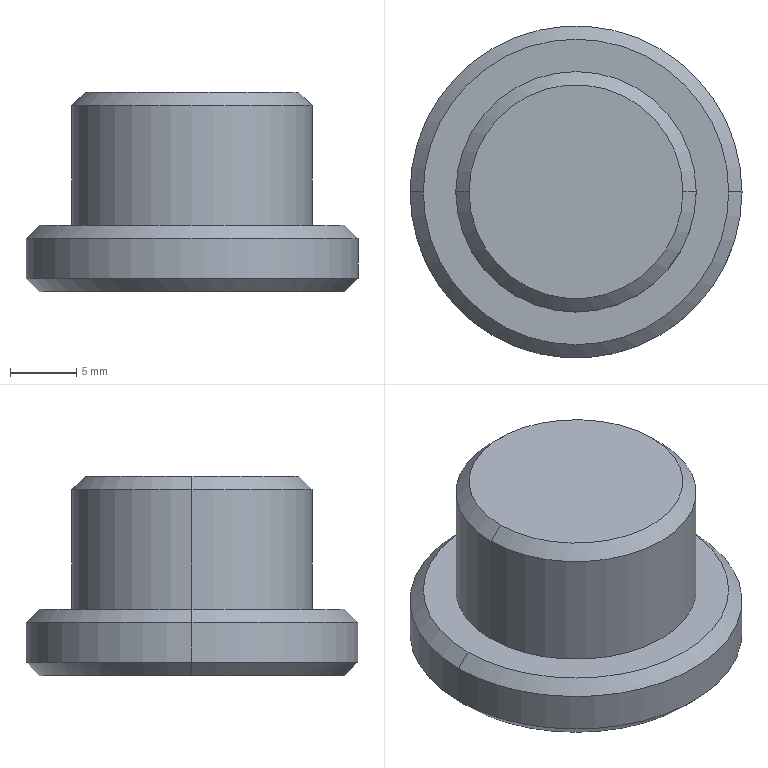Part | SolidWorks | features Chamfer 1, Revolution 1 | 1 solid | 13 faces | box 25 x 25 x 15 mm | volume 4924 mm3 | cone 6 | cylinder 4 | plane 3 | commonest cylinder face diameters 18.1 x2 25 x2
STEP:
#1=CARTESIAN_POINT('',(8.05,0.,0.));
#2=VERTEX_POINT('',#1);
#3=CARTESIAN_POINT('',(-8.05,0.,0.));
#4=VERTEX_POINT('',#3);
#5=CARTESIAN_POINT('',(0.,0.,0.));
#6=DIRECTION('',(0.,0.,1.));
#7=DIRECTION('',(-1.,0.,0.));
#8=AXIS2_PLACEMENT_3D('',#5,#6,#7);
#9=CIRCLE('',#8,8.05);
#10=EDGE_CURVE('',#2,#4,#9,.T.);
#11=ORIENTED_EDGE('',*,*,#10,.F.);
#12=CARTESIAN_POINT('',(9.05,0.,-1.));
#13=VERTEX_POINT('',#12);
#14=CARTESIAN_POINT('',(8.05,0.,0.));
#15=DIRECTION('',(0.7071,0.,-0.7071));
#16=VECTOR('',#15,1000.);
#17=LINE('',#14,#16);
#18=EDGE_CURVE('',#2,#13,#17,.T.);
#19=ORIENTED_EDGE('',*,*,#18,.T.);
#20=CARTESIAN_POINT('',(-9.05,0.,-1.));
#21=VERTEX_POINT('',#20);
#22=CARTESIAN_POINT('',(0.,0.,-1.));
#23=DIRECTION('',(0.,0.,-1.));
#24=DIRECTION('',(-1.,0.,0.));
#25=AXIS2_PLACEMENT_3D('',#22,#23,#24);
#26=CIRCLE('',#25,9.05);
#27=EDGE_CURVE('',#21,#13,#26,.T.);
#28=ORIENTED_EDGE('',*,*,#27,.F.);
#29=CARTESIAN_POINT('',(-8.05,0.,0.));
#30=DIRECTION('',(-0.7071,0.,-0.7071));
#31=VECTOR('',#30,1000.);
#32=LINE('',#29,#31);
#33=EDGE_CURVE('',#4,#21,#32,.T.);
#34=ORIENTED_EDGE('',*,*,#33,.F.);
#35=EDGE_LOOP('',(#11,#19,#28,#34));
#36=FACE_OUTER_BOUND('',#35,.T.);
#37=CARTESIAN_POINT('',(0.,0.,0.));
#38=DIRECTION('',(0.,0.,-1.));
#39=DIRECTION('',(-1.,0.,0.));
#40=AXIS2_PLACEMENT_3D('',#37,#38,#39);
#41=CONICAL_SURFACE('',#40,8.05,0.7854);
#42=ADVANCED_FACE('',(#36),#41,.T.);
#43=CARTESIAN_POINT('',(11.5,0.,-10.));
#44=VERTEX_POINT('',#43);
#45=CARTESIAN_POINT('',(-11.5,0.,-10.));
#46=VERTEX_POINT('',#45);
#47=CARTESIAN_POINT('',(0.,0.,-10.));
#48=DIRECTION('',(0.,0.,1.));
#49=DIRECTION('',(-1.,0.,0.));
#50=AXIS2_PLACEMENT_3D('',#47,#48,#49);
#51=CIRCLE('',#50,11.5);
#52=EDGE_CURVE('',#44,#46,#51,.T.);
#53=ORIENTED_EDGE('',*,*,#52,.F.);
#54=CARTESIAN_POINT('',(12.5,0.,-11.));
#55=VERTEX_POINT('',#54);
#56=CARTESIAN_POINT('',(11.5,0.,-10.));
#57=DIRECTION('',(0.7071,0.,-0.7071));
#58=VECTOR('',#57,1000.);
#59=LINE('',#56,#58);
#60=EDGE_CURVE('',#44,#55,#59,.T.);
#61=ORIENTED_EDGE('',*,*,#60,.T.);
#62=CARTESIAN_POINT('',(-12.5,0.,-11.));
#63=VERTEX_POINT('',#62);
#64=CARTESIAN_POINT('',(0.,0.,-11.));
#65=DIRECTION('',(0.,0.,-1.));
#66=DIRECTION('',(-1.,0.,0.));
#67=AXIS2_PLACEMENT_3D('',#64,#65,#66);
#68=CIRCLE('',#67,12.5);
#69=EDGE_CURVE('',#63,#55,#68,.T.);
#70=ORIENTED_EDGE('',*,*,#69,.F.);
#71=CARTESIAN_POINT('',(-11.5,0.,-10.));
#72=DIRECTION('',(-0.7071,0.,-0.7071));
#73=VECTOR('',#72,1000.);
#74=LINE('',#71,#73);
#75=EDGE_CURVE('',#46,#63,#74,.T.);
#76=ORIENTED_EDGE('',*,*,#75,.F.);
#77=EDGE_LOOP('',(#53,#61,#70,#76));
#78=FACE_OUTER_BOUND('',#77,.T.);
#79=CARTESIAN_POINT('',(0.,0.,-10.));
#80=DIRECTION('',(0.,0.,-1.));
#81=DIRECTION('',(-1.,0.,0.));
#82=AXIS2_PLACEMENT_3D('',#79,#80,#81);
#83=CONICAL_SURFACE('',#82,11.5,0.7854);
#84=ADVANCED_FACE('',(#78),#83,.T.);
#85=CARTESIAN_POINT('',(-11.5,0.,-15.));
#86=VERTEX_POINT('',#85);
#87=CARTESIAN_POINT('',(11.5,0.,-15.));
#88=VERTEX_POINT('',#87);
#89=CARTESIAN_POINT('',(0.,0.,-15.));
#90=DIRECTION('',(0.,0.,-1.));
#91=DIRECTION('',(1.,0.,0.));
#92=AXIS2_PLACEMENT_3D('',#89,#90,#91);
#93=CIRCLE('',#92,11.5);
#94=EDGE_CURVE('',#86,#88,#93,.T.);
#95=ORIENTED_EDGE('',*,*,#94,.F.);
#96=CARTESIAN_POINT('',(-12.5,0.,-14.));
#97=VERTEX_POINT('',#96);
#98=CARTESIAN_POINT('',(-12.5,0.,-14.));
#99=DIRECTION('',(-0.7071,0.,0.7071));
#100=VECTOR('',#99,1000.);
#101=LINE('',#98,#100);
#102=EDGE_CURVE('',#86,#97,#101,.T.);
#103=ORIENTED_EDGE('',*,*,#102,.T.);
#104=CARTESIAN_POINT('',(12.5,0.,-14.));
#105=VERTEX_POINT('',#104);
#106=CARTESIAN_POINT('',(0.,0.,-14.));
#107=DIRECTION('',(0.,0.,1.));
#108=DIRECTION('',(1.,0.,0.));
#109=AXIS2_PLACEMENT_3D('',#106,#107,#108);
#110=CIRCLE('',#109,12.5);
#111=EDGE_CURVE('',#105,#97,#110,.T.);
#112=ORIENTED_EDGE('',*,*,#111,.F.);
#113=CARTESIAN_POINT('',(12.5,0.,-14.));
#114=DIRECTION('',(0.7071,0.,0.7071));
#115=VECTOR('',#114,1000.);
#116=LINE('',#113,#115);
#117=EDGE_CURVE('',#88,#105,#116,.T.);
#118=ORIENTED_EDGE('',*,*,#117,.F.);
#119=EDGE_LOOP('',(#95,#103,#112,#118));
#120=FACE_OUTER_BOUND('',#119,.T.);
#121=CARTESIAN_POINT('',(0.,0.,-14.));
#122=DIRECTION('',(0.,0.,1.));
#123=DIRECTION('',(1.,0.,0.));
#124=AXIS2_PLACEMENT_3D('',#121,#122,#123);
#125=CONICAL_SURFACE('',#124,12.5,0.7854);
#126=ADVANCED_FACE('',(#120),#125,.T.);
#127=CARTESIAN_POINT('',(9.05,0.,-10.));
#128=VERTEX_POINT('',#127);
#129=CARTESIAN_POINT('',(-9.05,0.,-10.));
#130=VERTEX_POINT('',#129);
#131=CARTESIAN_POINT('',(0.,0.,-10.));
#132=DIRECTION('',(0.,0.,1.));
#133=DIRECTION('',(1.,0.,0.));
#134=AXIS2_PLACEMENT_3D('',#131,#132,#133);
#135=CIRCLE('',#134,9.05);
#136=EDGE_CURVE('',#128,#130,#135,.T.);
#137=ORIENTED_EDGE('',*,*,#136,.T.);
#138=CARTESIAN_POINT('',(-9.05,0.,0.));
#139=DIRECTION('',(0.,0.,1.));
#140=VECTOR('',#139,1000.);
#141=LINE('',#138,#140);
#142=EDGE_CURVE('',#130,#21,#141,.T.);
#143=ORIENTED_EDGE('',*,*,#142,.T.);
#144=ORIENTED_EDGE('',*,*,#27,.T.);
#145=CARTESIAN_POINT('',(9.05,0.,0.));
#146=DIRECTION('',(0.,0.,1.));
#147=VECTOR('',#146,1000.);
#148=LINE('',#145,#147);
#149=EDGE_CURVE('',#128,#13,#148,.T.);
#150=ORIENTED_EDGE('',*,*,#149,.F.);
#151=EDGE_LOOP('',(#137,#143,#144,#150));
#152=FACE_OUTER_BOUND('',#151,.T.);
#153=CARTESIAN_POINT('',(0.,0.,0.));
#154=DIRECTION('',(0.,0.,1.));
#155=DIRECTION('',(1.,0.,0.));
#156=AXIS2_PLACEMENT_3D('',#153,#154,#155);
#157=CYLINDRICAL_SURFACE('',#156,9.05);
#158=ADVANCED_FACE('',(#152),#157,.T.);
#159=ORIENTED_EDGE('',*,*,#111,.T.);
#160=CARTESIAN_POINT('',(-12.5,0.,0.));
#161=DIRECTION('',(0.,0.,1.));
#162=VECTOR('',#161,1000.);
#163=LINE('',#160,#162);
#164=EDGE_CURVE('',#97,#63,#163,.T.);
#165=ORIENTED_EDGE('',*,*,#164,.T.);
#166=ORIENTED_EDGE('',*,*,#69,.T.);
#167=CARTESIAN_POINT('',(12.5,0.,0.));
#168=DIRECTION('',(0.,0.,1.));
#169=VECTOR('',#168,1000.);
#170=LINE('',#167,#169);
#171=EDGE_CURVE('',#105,#55,#170,.T.);
#172=ORIENTED_EDGE('',*,*,#171,.F.);
#173=EDGE_LOOP('',(#159,#165,#166,#172));
#174=FACE_OUTER_BOUND('',#173,.T.);
#175=CARTESIAN_POINT('',(0.,0.,0.));
#176=DIRECTION('',(0.,0.,1.));
#177=DIRECTION('',(1.,0.,0.));
#178=AXIS2_PLACEMENT_3D('',#175,#176,#177);
#179=CYLINDRICAL_SURFACE('',#178,12.5);
#180=ADVANCED_FACE('',(#174),#179,.T.);
#181=CARTESIAN_POINT('',(0.,0.,-15.));
#182=DIRECTION('',(0.,0.,-1.));
#183=DIRECTION('',(1.,0.,0.));
#184=AXIS2_PLACEMENT_3D('',#181,#182,#183);
#185=CIRCLE('',#184,11.5);
#186=EDGE_CURVE('',#88,#86,#185,.T.);
#187=ORIENTED_EDGE('',*,*,#186,.T.);
#188=ORIENTED_EDGE('',*,*,#94,.T.);
#189=EDGE_LOOP('',(#187,#188));
#190=FACE_OUTER_BOUND('',#189,.T.);
#191=CARTESIAN_POINT('',(0.,0.,-15.));
#192=DIRECTION('',(0.,0.,1.));
#193=DIRECTION('',(1.,0.,0.));
#194=AXIS2_PLACEMENT_3D('',#191,#192,#193);
#195=PLANE('',#194);
#196=ADVANCED_FACE('',(#190),#195,.F.);
#197=ORIENTED_EDGE('',*,*,#164,.F.);
#198=CARTESIAN_POINT('',(0.,0.,-14.));
#199=DIRECTION('',(0.,0.,1.));
#200=DIRECTION('',(1.,0.,0.));
#201=AXIS2_PLACEMENT_3D('',#198,#199,#200);
#202=CIRCLE('',#201,12.5);
#203=EDGE_CURVE('',#97,#105,#202,.T.);
#204=ORIENTED_EDGE('',*,*,#203,.T.);
#205=ORIENTED_EDGE('',*,*,#171,.T.);
#206=CARTESIAN_POINT('',(0.,0.,-11.));
#207=DIRECTION('',(0.,0.,-1.));
#208=DIRECTION('',(-1.,0.,0.));
#209=AXIS2_PLACEMENT_3D('',#206,#207,#208);
#210=CIRCLE('',#209,12.5);
#211=EDGE_CURVE('',#55,#63,#210,.T.);
#212=ORIENTED_EDGE('',*,*,#211,.T.);
#213=EDGE_LOOP('',(#197,#204,#205,#212));
#214=FACE_OUTER_BOUND('',#213,.T.);
#215=CARTESIAN_POINT('',(0.,0.,0.));
#216=DIRECTION('',(0.,0.,1.));
#217=DIRECTION('',(1.,0.,0.));
#218=AXIS2_PLACEMENT_3D('',#215,#216,#217);
#219=CYLINDRICAL_SURFACE('',#218,12.5);
#220=ADVANCED_FACE('',(#214),#219,.T.);
#221=CARTESIAN_POINT('',(0.,0.,-10.));
#222=DIRECTION('',(0.,0.,1.));
#223=DIRECTION('',(-1.,0.,0.));
#224=AXIS2_PLACEMENT_3D('',#221,#222,#223);
#225=CIRCLE('',#224,11.5);
#226=EDGE_CURVE('',#46,#44,#225,.T.);
#227=ORIENTED_EDGE('',*,*,#226,.T.);
#228=ORIENTED_EDGE('',*,*,#52,.T.);
#229=EDGE_LOOP('',(#227,#228));
#230=FACE_OUTER_BOUND('',#229,.T.);
#231=ORIENTED_EDGE('',*,*,#136,.F.);
#232=CARTESIAN_POINT('',(0.,0.,-10.));
#233=DIRECTION('',(0.,0.,1.));
#234=DIRECTION('',(1.,0.,0.));
#235=AXIS2_PLACEMENT_3D('',#232,#233,#234);
#236=CIRCLE('',#235,9.05);
#237=EDGE_CURVE('',#130,#128,#236,.T.);
#238=ORIENTED_EDGE('',*,*,#237,.F.);
#239=EDGE_LOOP('',(#231,#238));
#240=FACE_BOUND('',#239,.T.);
#241=CARTESIAN_POINT('',(0.,12.5,-10.));
#242=DIRECTION('',(0.,0.,-1.));
#243=DIRECTION('',(-1.,0.,0.));
#244=AXIS2_PLACEMENT_3D('',#241,#242,#243);
#245=PLANE('',#244);
#246=ADVANCED_FACE('',(#230,#240),#245,.F.);
#247=ORIENTED_EDGE('',*,*,#142,.F.);
#248=ORIENTED_EDGE('',*,*,#237,.T.);
#249=ORIENTED_EDGE('',*,*,#149,.T.);
#250=CARTESIAN_POINT('',(0.,0.,-1.));
#251=DIRECTION('',(0.,0.,-1.));
#252=DIRECTION('',(-1.,0.,0.));
#253=AXIS2_PLACEMENT_3D('',#250,#251,#252);
#254=CIRCLE('',#253,9.05);
#255=EDGE_CURVE('',#13,#21,#254,.T.);
#256=ORIENTED_EDGE('',*,*,#255,.T.);
#257=EDGE_LOOP('',(#247,#248,#249,#256));
#258=FACE_OUTER_BOUND('',#257,.T.);
#259=CARTESIAN_POINT('',(0.,0.,0.));
#260=DIRECTION('',(0.,0.,1.));
#261=DIRECTION('',(1.,0.,0.));
#262=AXIS2_PLACEMENT_3D('',#259,#260,#261);
#263=CYLINDRICAL_SURFACE('',#262,9.05);
#264=ADVANCED_FACE('',(#258),#263,.T.);
#265=CARTESIAN_POINT('',(0.,0.,0.));
#266=DIRECTION('',(0.,0.,1.));
#267=DIRECTION('',(-1.,0.,0.));
#268=AXIS2_PLACEMENT_3D('',#265,#266,#267);
#269=CIRCLE('',#268,8.05);
#270=EDGE_CURVE('',#4,#2,#269,.T.);
#271=ORIENTED_EDGE('',*,*,#270,.T.);
#272=ORIENTED_EDGE('',*,*,#10,.T.);
#273=EDGE_LOOP('',(#271,#272));
#274=FACE_OUTER_BOUND('',#273,.T.);
#275=CARTESIAN_POINT('',(0.,9.05,0.));
#276=DIRECTION('',(0.,0.,-1.));
#277=DIRECTION('',(-1.,0.,0.));
#278=AXIS2_PLACEMENT_3D('',#275,#276,#277);
#279=PLANE('',#278);
#280=ADVANCED_FACE('',(#274),#279,.F.);
#281=ORIENTED_EDGE('',*,*,#102,.F.);
#282=ORIENTED_EDGE('',*,*,#186,.F.);
#283=ORIENTED_EDGE('',*,*,#117,.T.);
#284=ORIENTED_EDGE('',*,*,#203,.F.);
#285=EDGE_LOOP('',(#281,#282,#283,#284));
#286=FACE_OUTER_BOUND('',#285,.T.);
#287=CARTESIAN_POINT('',(0.,0.,-14.));
#288=DIRECTION('',(0.,0.,1.));
#289=DIRECTION('',(1.,0.,0.));
#290=AXIS2_PLACEMENT_3D('',#287,#288,#289);
#291=CONICAL_SURFACE('',#290,12.5,0.7854);
#292=ADVANCED_FACE('',(#286),#291,.T.);
#293=ORIENTED_EDGE('',*,*,#60,.F.);
#294=ORIENTED_EDGE('',*,*,#226,.F.);
#295=ORIENTED_EDGE('',*,*,#75,.T.);
#296=ORIENTED_EDGE('',*,*,#211,.F.);
#297=EDGE_LOOP('',(#293,#294,#295,#296));
#298=FACE_OUTER_BOUND('',#297,.T.);
#299=CARTESIAN_POINT('',(0.,0.,-10.));
#300=DIRECTION('',(0.,0.,-1.));
#301=DIRECTION('',(-1.,0.,0.));
#302=AXIS2_PLACEMENT_3D('',#299,#300,#301);
#303=CONICAL_SURFACE('',#302,11.5,0.7854);
#304=ADVANCED_FACE('',(#298),#303,.T.);
#305=ORIENTED_EDGE('',*,*,#18,.F.);
#306=ORIENTED_EDGE('',*,*,#270,.F.);
#307=ORIENTED_EDGE('',*,*,#33,.T.);
#308=ORIENTED_EDGE('',*,*,#255,.F.);
#309=EDGE_LOOP('',(#305,#306,#307,#308));
#310=FACE_OUTER_BOUND('',#309,.T.);
#311=CARTESIAN_POINT('',(0.,0.,0.));
#312=DIRECTION('',(0.,0.,-1.));
#313=DIRECTION('',(-1.,0.,0.));
#314=AXIS2_PLACEMENT_3D('',#311,#312,#313);
#315=CONICAL_SURFACE('',#314,8.05,0.7854);
#316=ADVANCED_FACE('',(#310),#315,.T.);
#317=CLOSED_SHELL('',(#42,#84,#126,#158,#180,#196,#220,#246,#264,#280,#292,#304,#316));
#318=MANIFOLD_SOLID_BREP('',#317);
#319=CARTESIAN_POINT('',(0.,0.,0.));
#320=DIRECTION('',(0.,0.,1.));
#321=DIRECTION('',(1.,0.,0.));
#322=AXIS2_PLACEMENT_3D('',#319,#320,#321);
#323=(LENGTH_UNIT()NAMED_UNIT(*)SI_UNIT(.MILLI.,.METRE.));
#324=UNCERTAINTY_MEASURE_WITH_UNIT(LENGTH_MEASURE(0.00001),#323,'','');
#325=(NAMED_UNIT(*)PLANE_ANGLE_UNIT()SI_UNIT($,.RADIAN.));
#326=(NAMED_UNIT(*)SI_UNIT($,.STERADIAN.)SOLID_ANGLE_UNIT());
#327=(GEOMETRIC_REPRESENTATION_CONTEXT(3)GLOBAL_UNCERTAINTY_ASSIGNED_CONTEXT((#324))GLOBAL_UNIT_ASSIGNED_CONTEXT((#323,#325,#326))REPRESENTATION_CONTEXT('',''));
#328=ADVANCED_BREP_SHAPE_REPRESENTATION('',(#318,#322),#327);